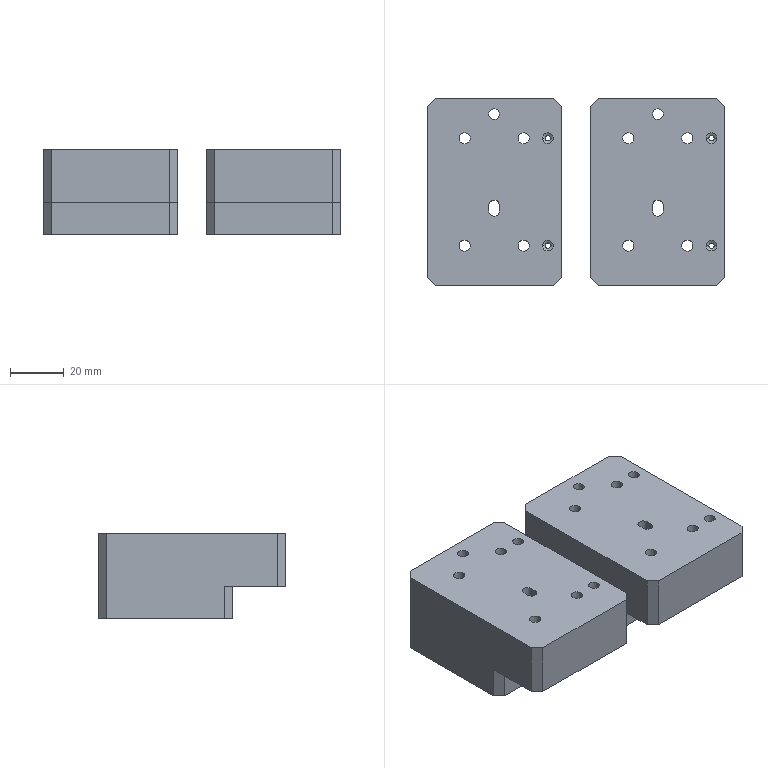Part | 2 solids | 112 faces | box 111 x 70 x 32 mm | volume 192401 mm3 | cylinder 56 | plane 32 | cone 24 | commonest cylinder face diameters 3.3 x16 4 x16 4.2 x16 2 x8